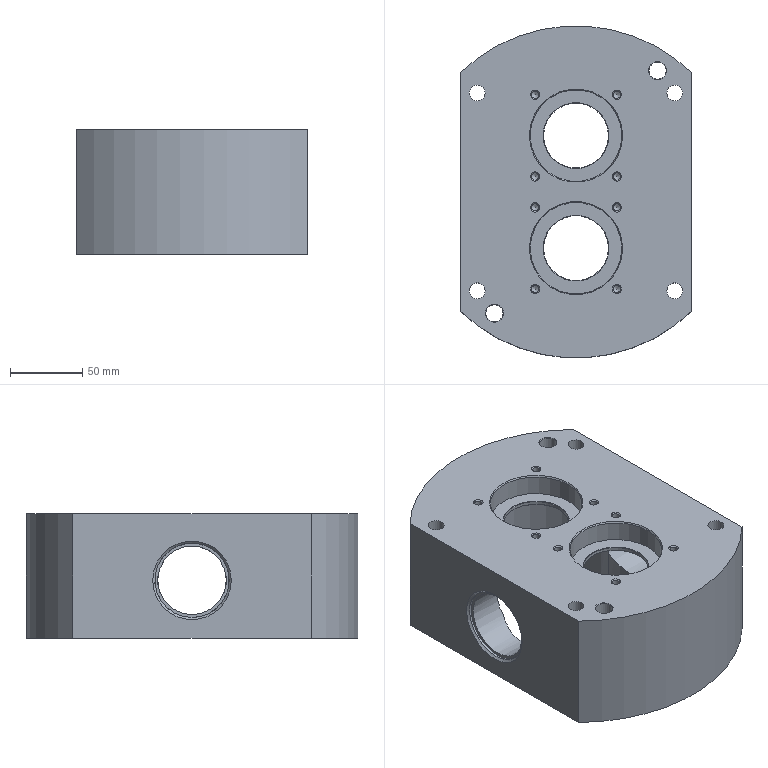NC program | NX | posted with a generic post | part box 160 x 230 x 86 mm
Lines 1876 to 2142 of 2142:
(ZLEVEL_PROFILE , TOOL : D10JING)
N3714 T11 M6
N3716 G54
N3718 G17 G0 G90 X-50.078 Y-10.841 B0. C0. S5000 M3
N3720 G43 Z30. H11
N3722 Z-16.
N3724 G94 G1 Z-18. F1250.
N3726 X-50.368 Y-12.67
N3728 G3 X-50.009 Y-13.603 R1.
N3730 G1 X-50.004 Y-13.607
N3732 G3 X-25.393 Y-11.004 R17.5
N3734 X-50.009 Y-13.603 R-17.5
N3736 X-49.021 Y-13.76 R1.
N3738 G1 X-47.292 Y-13.095
N3740 Z-16.
N3742 G0 Z30.
N3744 X27.919 Y-10.838
N3746 Z-16.
N3748 G1 Z-18.
N3750 X27.63 Y-12.669
N3752 G3 X27.989 Y-13.602 R1.
N3754 G1 X27.999 Y-13.61
N3756 G3 X52.61 Y-11.001 R17.5
N3758 X27.989 Y-13.602 R-17.5
N3760 X28.977 Y-13.758 R1.
N3762 G1 X30.706 Y-13.094
N3764 Z-16.
N3766 G0 Z30.
N3768 M5
(PLANAR_MILL_COPY_COPY , TOOL : D6A45)
N3770 T07 M6
N3772 G54
N3774 G17 G0 G90 X66.379 Y-71.028 B0. C0. S7500 M3
N3776 G43 Z30. H7
N3778 Z1.5
N3780 G94 G1 Z-1.5 F1250.
N3782 X67.734 Y-72.643
N3784 G3 X68.5 Y-73. R1.
N3786 X73. Y-68.5 R4.5
N3788 X68.5 Y-73. R-4.5
N3790 X69.266 Y-72.643 R1.
N3792 G1 X70.621 Y-71.028
N3794 Z1.5
N3796 G0 Z30.
N3798 X82.099 Y-59.79
N3800 Z1.5
N3802 G1 Z-1.5
N3804 X83.234 Y-61.143
N3806 G3 X84. Y-61.5 R1.
N3808 X89. Y-56.5 R5.
N3810 X84. Y-61.5 R-5.
N3812 X84.766 Y-61.143 R1.
N3814 G1 X85.901 Y-59.79
N3816 Z1.5
N3818 G0 Z30.
N3820 X67.533 Y-28.451
N3822 Z1.5
N3824 G1 Z-1.5
N3826 X68.427 Y-29.05
N3828 G3 X68.784 Y-28.284 R1.
N3830 X67.284 Y-26.784 R1.5
N3832 X68.784 Y-28.284 R-1.5
N3834 X68.427 Y-27.518 R1.
N3836 G1 X67.533 Y-28.117
N3838 Z1.5
N3840 G0 Z30.
N3842 X10.549 Y-28.533
N3844 Z1.5
N3846 G1 Z-1.5
N3848 X9.95 Y-29.427
N3850 G3 X10.716 Y-29.784 R1.
N3852 X12.216 Y-28.284 R1.5
N3854 X10.716 Y-29.784 R-1.5
N3856 X11.482 Y-29.427 R1.
N3858 G1 X10.883 Y-28.533
N3860 Z1.5
N3862 G0 Z30.
N3864 X-10.883
N3866 Z1.5
N3868 G1 Z-1.5
N3870 X-11.482 Y-29.427
N3872 G3 X-10.716 Y-29.784 R1.
N3874 X-9.216 Y-28.284 R1.5
N3876 X-10.716 Y-29.784 R-1.5
N3878 X-9.95 Y-29.427 R1.
N3880 G1 X-10.549 Y-28.533
N3882 Z1.5
N3884 G0 Z30.
N3886 X-70.621 Y-71.028
N3888 Z1.5
N3890 G1 Z-1.5
N3892 X-69.266 Y-72.643
N3894 G3 X-68.5 Y-73. R1.
N3896 X-64. Y-68.5 R4.5
N3898 X-68.5 Y-73. R-4.5
N3900 X-67.734 Y-72.643 R1.
N3902 G1 X-66.379 Y-71.028
N3904 Z1.5
N3906 G0 Z30.
N3908 X-67.533 Y-28.117
N3910 Z1.5
N3912 G1 Z-1.5
N3914 X-68.427 Y-27.518
N3916 G3 X-68.784 Y-28.284 R1.
N3918 X-67.284 Y-29.784 R1.5
N3920 X-68.784 Y-28.284 R-1.5
N3922 X-68.427 Y-29.05 R1.
N3924 G1 X-67.533 Y-28.451
N3926 Z1.5
N3928 G0 Z30.
N3930 X-68.512 Y1.505
N3932 Z1.5
N3934 G1 Z-1.5
N3936 X-69.393 Y0.766
N3938 G3 X-69.75 Y0. R1.
N3940 X-39. Y-30.75 R30.75
N3942 X-69.75 Y0. R-30.75
N3944 X-69.393 Y-0.766 R1.
N3946 G1 X-68.512 Y-1.505
N3948 Z1.5
N3950 G0 Z30.
N3952 X-67.533 Y28.451
N3954 Z1.5
N3956 G1 Z-1.5
N3958 X-68.427 Y29.05
N3960 G3 X-68.784 Y28.284 R1.
N3962 X-67.284 Y26.784 R1.5
N3964 X-68.784 Y28.284 R-1.5
N3966 X-68.427 Y27.518 R1.
N3968 G1 X-67.533 Y28.117
N3970 Z1.5
N3972 G0 Z30.
N3974 X-82.099 Y59.79
N3976 Z1.5
N3978 G1 Z-1.5
N3980 X-83.234 Y61.143
N3982 G3 X-84. Y61.5 R1.
N3984 X-89. Y56.5 R5.
N3986 X-84. Y61.5 R-5.
N3988 X-84.766 Y61.143 R1.
N3990 G1 X-85.901 Y59.79
N3992 Z1.5
N3994 G0 Z30.
N3996 X-66.379 Y71.028
N3998 Z1.5
N4000 G1 Z-1.5
N4002 X-67.734 Y72.643
N4004 G3 X-68.5 Y73. R1.
N4006 X-73. Y68.5 R4.5
N4008 X-68.5 Y73. R-4.5
N4010 X-69.266 Y72.643 R1.
N4012 G1 X-70.621 Y71.028
N4014 Z1.5
N4016 G0 Z30.
N4018 X-10.549 Y28.533
N4020 Z1.5
N4022 G1 Z-1.5
N4024 X-9.95 Y29.427
N4026 G3 X-10.716 Y29.784 R1.
N4028 X-12.216 Y28.284 R1.5
N4030 X-10.716 Y29.784 R-1.5
N4032 X-11.482 Y29.427 R1.
N4034 G1 X-10.883 Y28.533
N4036 Z1.5
N4038 G0 Z30.
N4040 X10.883
N4042 Z1.5
N4044 G1 Z-1.5
N4046 X11.482 Y29.427
N4048 G3 X10.716 Y29.784 R1.
N4050 X9.216 Y28.284 R1.5
N4052 X10.716 Y29.784 R-1.5
N4054 X9.95 Y29.427 R1.
N4056 G1 X10.549 Y28.533
N4058 Z1.5
N4060 G0 Z30.
N4062 X40.505 Y29.512
N4064 Z1.5
N4066 G1 Z-1.5
N4068 X39.766 Y30.393
N4070 G3 X39. Y30.75 R1.
N4072 X8.25 Y0. R30.75
N4074 X39. Y30.75 R-30.75
N4076 X38.234 Y30.393 R1.
N4078 G1 X37.495 Y29.512
N4080 Z1.5
N4082 G0 Z30.
N4084 X67.533 Y28.117
N4086 Z1.5
N4088 G1 Z-1.5
N4090 X68.427 Y27.518
N4092 G3 X68.784 Y28.284 R1.
N4094 X67.284 Y29.784 R1.5
N4096 X68.784 Y28.284 R-1.5
N4098 X68.427 Y29.05 R1.
N4100 G1 X67.533 Y28.451
N4102 Z1.5
N4104 G0 Z30.
N4106 X70.621 Y71.028
N4108 Z1.5
N4110 G1 Z-1.5
N4112 X69.266 Y72.643
N4114 G3 X68.5 Y73. R1.
N4116 X64. Y68.5 R4.5
N4118 X68.5 Y73. R-4.5
N4120 X67.734 Y72.643 R1.
N4122 G1 X66.379 Y71.028
N4124 Z1.5
N4126 G0 Z30.
(PLANAR_MILL_COPY_COPY_COPY , TOOL : D6A45)
N4128 X-40.522 Y-20.042
N4130 Z-13.5
N4132 G1 Z-16.5
N4134 X-39.766 Y-20.943
N4136 G3 X-39. Y-21.3 R1.
N4138 X-17.7 Y0. R21.3
N4140 X-39. Y-21.3 R-21.3
N4142 X-38.234 Y-20.943 R1.
N4144 G1 X-37.478 Y-20.042
N4146 Z-13.5
N4148 G0 Z30.
N4150 X37.478
N4152 Z-13.5
N4154 G1 Z-16.5
N4156 X38.234 Y-20.943
N4158 G3 X39. Y-21.3 R1.
N4160 X60.3 Y0. R21.3
N4162 X39. Y-21.3 R-21.3
N4164 X39.766 Y-20.943 R1.
N4166 G1 X40.522 Y-20.042
N4168 Z-13.5
N4170 G0 Z30.
N4172 M5
(刀补 , TOOL : D10JING)
N4174 T11 M6
N4176 G54
N4178 G17 G0 G90 X-42.434 Y-23.248 B0. C0. S5000 M3
N4180 G43 Z30. H11
N4182 Z-15.
N4184 G41 G94 G1 X-42.448 Y-23.347 F1000. D11
N4186 G3 X-39. Y-26.7 R3.449
N4188 X-12.3 Y0. R26.7
N4190 X-39. Y-26.7 R-26.7
N4192 X-35.552 Y-23.347 R3.449
N4194 G40
N4196 G1 X-35.566 Y-23.248
N4198 G0 Z30.
N4200 X35.566
N4202 Z-15.
N4204 G41 G1 X35.552 Y-23.347
N4206 G3 X39. Y-26.7 R3.449
N4208 X65.7 Y0. R26.7
N4210 X39. Y-26.7 R-26.7
N4212 X42.448 Y-23.347 R3.449
N4214 G40
N4216 G1 X42.434 Y-23.248
N4218 G0 Z30.
N4220 M5
N4222 M2